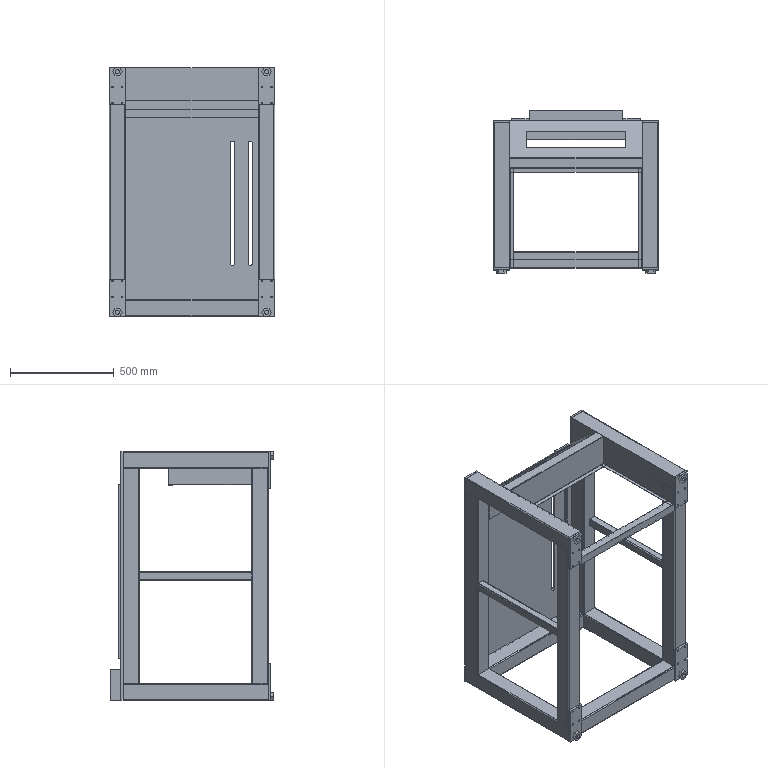Part | STEP file | Frame | 29 solids | 441 faces | box 800 x 785 x 1200 mm | volume 26873154 mm3 | plane 302 | cylinder 139 | commonest cylinder face diameters 6.8 x64 10 x40 20 x17 25 x8 1 x5 4 x5